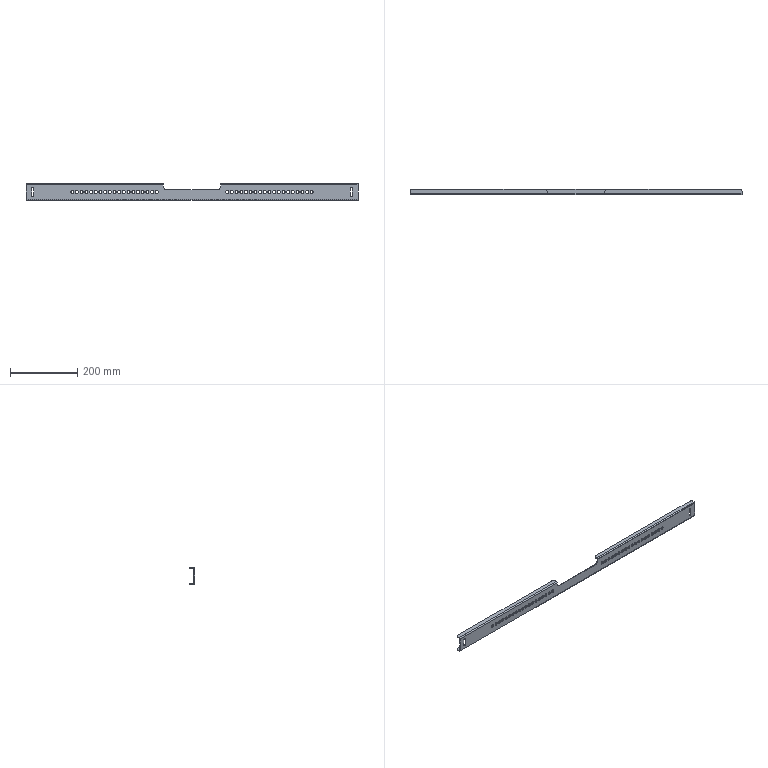Part | SolidWorks | features ICE 3, Fillet 2, EdgeFlange 1, FlatPattern 1, HoleWzd 1, LPattern 1, MirrorPattern 1, SMBaseFlange 1, SheetMetal 1 | 1 solid | 128 faces | box 990 x 15 x 50 mm | volume 130512 mm3 | cylinder 96 | plane 32 | commonest cylinder face diameters 9.2 x76 7 x6 10 x4 20 x4 2.54 x3 6.54 x3